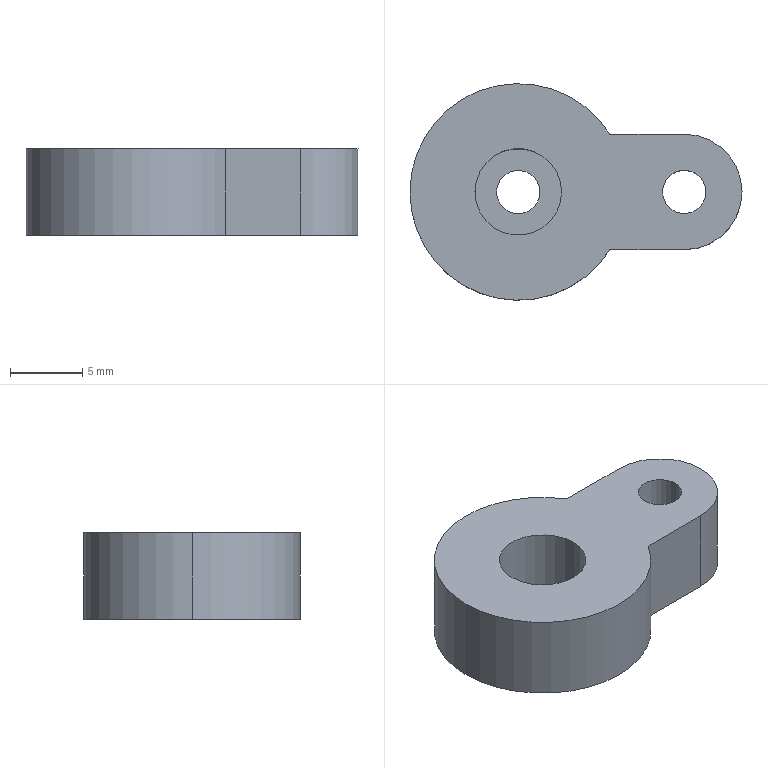Part | SolidWorks | features BaseBody 1, Cut 1 | 1 solid | 15 faces | box 23 x 15 x 6 mm | volume 1241 mm3 | cylinder 10 | plane 5 | commonest cylinder face diameters 3 x4 6 x2 8 x2 15 x2
STEP:
#1=CARTESIAN_POINT('',(-4.04,16.034,1.5));
#2=VERTEX_POINT('',#1);
#3=CARTESIAN_POINT('',(1.96,16.034,1.5));
#4=VERTEX_POINT('',#3);
#5=CARTESIAN_POINT('',(-1.04,16.034,1.5));
#6=DIRECTION('',(0.,0.,1.));
#7=DIRECTION('',(1.,0.,0.));
#8=AXIS2_PLACEMENT_3D('',#5,#6,#7);
#9=CIRCLE('',#8,3.);
#10=EDGE_CURVE('',#2,#4,#9,.T.);
#11=ORIENTED_EDGE('',*,*,#10,.F.);
#12=CARTESIAN_POINT('',(-4.04,16.034,6.));
#13=VERTEX_POINT('',#12);
#14=CARTESIAN_POINT('',(-4.04,16.034,1.5));
#15=DIRECTION('',(0.,0.,1.));
#16=VECTOR('',#15,1000.);
#17=LINE('',#14,#16);
#18=EDGE_CURVE('',#2,#13,#17,.T.);
#19=ORIENTED_EDGE('',*,*,#18,.T.);
#20=CARTESIAN_POINT('',(1.96,16.034,6.));
#21=VERTEX_POINT('',#20);
#22=CARTESIAN_POINT('',(-1.04,16.034,6.));
#23=DIRECTION('',(0.,0.,1.));
#24=DIRECTION('',(1.,0.,0.));
#25=AXIS2_PLACEMENT_3D('',#22,#23,#24);
#26=CIRCLE('',#25,3.);
#27=EDGE_CURVE('',#13,#21,#26,.T.);
#28=ORIENTED_EDGE('',*,*,#27,.T.);
#29=CARTESIAN_POINT('',(1.96,16.034,1.5));
#30=DIRECTION('',(0.,0.,1.));
#31=VECTOR('',#30,1000.);
#32=LINE('',#29,#31);
#33=EDGE_CURVE('',#4,#21,#32,.T.);
#34=ORIENTED_EDGE('',*,*,#33,.F.);
#35=EDGE_LOOP('',(#11,#19,#28,#34));
#36=FACE_OUTER_BOUND('',#35,.T.);
#37=CARTESIAN_POINT('',(-1.04,16.034,1.5));
#38=DIRECTION('',(0.,0.,1.));
#39=DIRECTION('',(1.,0.,0.));
#40=AXIS2_PLACEMENT_3D('',#37,#38,#39);
#41=CYLINDRICAL_SURFACE('',#40,3.);
#42=ADVANCED_FACE('',(#36),#41,.F.);
#43=CARTESIAN_POINT('',(-2.54,16.034,1.5));
#44=VERTEX_POINT('',#43);
#45=CARTESIAN_POINT('',(0.46,16.034,1.5));
#46=VERTEX_POINT('',#45);
#47=CARTESIAN_POINT('',(-1.04,16.034,1.5));
#48=DIRECTION('',(0.,0.,-1.));
#49=DIRECTION('',(1.,0.,0.));
#50=AXIS2_PLACEMENT_3D('',#47,#48,#49);
#51=CIRCLE('',#50,1.5);
#52=EDGE_CURVE('',#44,#46,#51,.T.);
#53=ORIENTED_EDGE('',*,*,#52,.F.);
#54=CARTESIAN_POINT('',(-2.54,16.034,0.));
#55=VERTEX_POINT('',#54);
#56=CARTESIAN_POINT('',(-2.54,16.034,6.));
#57=DIRECTION('',(0.,0.,-1.));
#58=VECTOR('',#57,1000.);
#59=LINE('',#56,#58);
#60=EDGE_CURVE('',#44,#55,#59,.T.);
#61=ORIENTED_EDGE('',*,*,#60,.T.);
#62=CARTESIAN_POINT('',(0.46,16.034,0.));
#63=VERTEX_POINT('',#62);
#64=CARTESIAN_POINT('',(-1.04,16.034,0.));
#65=DIRECTION('',(0.,0.,1.));
#66=DIRECTION('',(1.,0.,0.));
#67=AXIS2_PLACEMENT_3D('',#64,#65,#66);
#68=CIRCLE('',#67,1.5);
#69=EDGE_CURVE('',#63,#55,#68,.T.);
#70=ORIENTED_EDGE('',*,*,#69,.F.);
#71=CARTESIAN_POINT('',(0.46,16.034,6.));
#72=DIRECTION('',(0.,0.,-1.));
#73=VECTOR('',#72,1000.);
#74=LINE('',#71,#73);
#75=EDGE_CURVE('',#46,#63,#74,.T.);
#76=ORIENTED_EDGE('',*,*,#75,.F.);
#77=EDGE_LOOP('',(#53,#61,#70,#76));
#78=FACE_OUTER_BOUND('',#77,.T.);
#79=CARTESIAN_POINT('',(-1.04,16.034,6.));
#80=DIRECTION('',(0.,0.,-1.));
#81=DIRECTION('',(-1.,0.,0.));
#82=AXIS2_PLACEMENT_3D('',#79,#80,#81);
#83=CYLINDRICAL_SURFACE('',#82,1.5);
#84=ADVANCED_FACE('',(#78),#83,.F.);
#85=CARTESIAN_POINT('',(-1.04,16.034,1.5));
#86=DIRECTION('',(0.,0.,-1.));
#87=DIRECTION('',(1.,0.,0.));
#88=AXIS2_PLACEMENT_3D('',#85,#86,#87);
#89=CIRCLE('',#88,1.5);
#90=EDGE_CURVE('',#46,#44,#89,.T.);
#91=ORIENTED_EDGE('',*,*,#90,.F.);
#92=ORIENTED_EDGE('',*,*,#75,.T.);
#93=CARTESIAN_POINT('',(-1.04,16.034,0.));
#94=DIRECTION('',(0.,0.,1.));
#95=DIRECTION('',(1.,0.,0.));
#96=AXIS2_PLACEMENT_3D('',#93,#94,#95);
#97=CIRCLE('',#96,1.5);
#98=EDGE_CURVE('',#55,#63,#97,.T.);
#99=ORIENTED_EDGE('',*,*,#98,.F.);
#100=ORIENTED_EDGE('',*,*,#60,.F.);
#101=EDGE_LOOP('',(#91,#92,#99,#100));
#102=FACE_OUTER_BOUND('',#101,.T.);
#103=CARTESIAN_POINT('',(-1.04,16.034,6.));
#104=DIRECTION('',(0.,0.,-1.));
#105=DIRECTION('',(-1.,0.,0.));
#106=AXIS2_PLACEMENT_3D('',#103,#104,#105);
#107=CYLINDRICAL_SURFACE('',#106,1.5);
#108=ADVANCED_FACE('',(#102),#107,.F.);
#109=CARTESIAN_POINT('',(14.46,16.034,0.));
#110=VERTEX_POINT('',#109);
#111=CARTESIAN_POINT('',(14.46,16.034,6.));
#112=VERTEX_POINT('',#111);
#113=CARTESIAN_POINT('',(14.46,16.034,-2.));
#114=DIRECTION('',(0.,0.,1.));
#115=VECTOR('',#114,1000.);
#116=LINE('',#113,#115);
#117=EDGE_CURVE('',#110,#112,#116,.T.);
#118=ORIENTED_EDGE('',*,*,#117,.F.);
#119=CARTESIAN_POINT('',(10.46,20.034,0.));
#120=VERTEX_POINT('',#119);
#121=CARTESIAN_POINT('',(10.46,16.034,0.));
#122=DIRECTION('',(0.,0.,-1.));
#123=DIRECTION('',(1.,0.,0.));
#124=AXIS2_PLACEMENT_3D('',#121,#122,#123);
#125=CIRCLE('',#124,4.);
#126=EDGE_CURVE('',#120,#110,#125,.T.);
#127=ORIENTED_EDGE('',*,*,#126,.F.);
#128=CARTESIAN_POINT('',(10.46,20.034,6.));
#129=VERTEX_POINT('',#128);
#130=CARTESIAN_POINT('',(10.46,20.034,6.));
#131=DIRECTION('',(0.,0.,-1.));
#132=VECTOR('',#131,1000.);
#133=LINE('',#130,#132);
#134=EDGE_CURVE('',#129,#120,#133,.T.);
#135=ORIENTED_EDGE('',*,*,#134,.F.);
#136=CARTESIAN_POINT('',(10.46,16.034,6.));
#137=DIRECTION('',(0.,0.,-1.));
#138=DIRECTION('',(1.,0.,0.));
#139=AXIS2_PLACEMENT_3D('',#136,#137,#138);
#140=CIRCLE('',#139,4.);
#141=EDGE_CURVE('',#129,#112,#140,.T.);
#142=ORIENTED_EDGE('',*,*,#141,.T.);
#143=EDGE_LOOP('',(#118,#127,#135,#142));
#144=FACE_OUTER_BOUND('',#143,.T.);
#145=CARTESIAN_POINT('',(10.46,16.034,-2.));
#146=DIRECTION('',(0.,0.,1.));
#147=DIRECTION('',(1.,0.,0.));
#148=AXIS2_PLACEMENT_3D('',#145,#146,#147);
#149=CYLINDRICAL_SURFACE('',#148,4.);
#150=ADVANCED_FACE('',(#144),#149,.T.);
#151=CARTESIAN_POINT('',(8.96,16.034,0.));
#152=VERTEX_POINT('',#151);
#153=CARTESIAN_POINT('',(8.96,16.034,6.));
#154=VERTEX_POINT('',#153);
#155=CARTESIAN_POINT('',(8.96,16.034,-4.));
#156=DIRECTION('',(0.,0.,1.));
#157=VECTOR('',#156,1000.);
#158=LINE('',#155,#157);
#159=EDGE_CURVE('',#152,#154,#158,.T.);
#160=ORIENTED_EDGE('',*,*,#159,.F.);
#161=CARTESIAN_POINT('',(11.96,16.034,0.));
#162=VERTEX_POINT('',#161);
#163=CARTESIAN_POINT('',(10.46,16.034,0.));
#164=DIRECTION('',(0.,0.,1.));
#165=DIRECTION('',(1.,0.,0.));
#166=AXIS2_PLACEMENT_3D('',#163,#164,#165);
#167=CIRCLE('',#166,1.5);
#168=EDGE_CURVE('',#162,#152,#167,.T.);
#169=ORIENTED_EDGE('',*,*,#168,.F.);
#170=CARTESIAN_POINT('',(11.96,16.034,6.));
#171=VERTEX_POINT('',#170);
#172=CARTESIAN_POINT('',(11.96,16.034,-4.));
#173=DIRECTION('',(0.,0.,1.));
#174=VECTOR('',#173,1000.);
#175=LINE('',#172,#174);
#176=EDGE_CURVE('',#162,#171,#175,.T.);
#177=ORIENTED_EDGE('',*,*,#176,.T.);
#178=CARTESIAN_POINT('',(10.46,16.034,6.));
#179=DIRECTION('',(0.,0.,1.));
#180=DIRECTION('',(1.,0.,0.));
#181=AXIS2_PLACEMENT_3D('',#178,#179,#180);
#182=CIRCLE('',#181,1.5);
#183=EDGE_CURVE('',#171,#154,#182,.T.);
#184=ORIENTED_EDGE('',*,*,#183,.T.);
#185=EDGE_LOOP('',(#160,#169,#177,#184));
#186=FACE_OUTER_BOUND('',#185,.T.);
#187=CARTESIAN_POINT('',(10.46,16.034,-4.));
#188=DIRECTION('',(0.,0.,1.));
#189=DIRECTION('',(1.,0.,0.));
#190=AXIS2_PLACEMENT_3D('',#187,#188,#189);
#191=CYLINDRICAL_SURFACE('',#190,1.5);
#192=ADVANCED_FACE('',(#186),#191,.F.);
#193=CARTESIAN_POINT('',(5.304,20.034,6.));
#194=VERTEX_POINT('',#193);
#195=CARTESIAN_POINT('',(22.96,20.034,6.));
#196=DIRECTION('',(-1.,0.,0.));
#197=VECTOR('',#196,1000.);
#198=LINE('',#195,#197);
#199=EDGE_CURVE('',#129,#194,#198,.T.);
#200=ORIENTED_EDGE('',*,*,#199,.F.);
#201=ORIENTED_EDGE('',*,*,#134,.T.);
#202=CARTESIAN_POINT('',(5.304,20.034,0.));
#203=VERTEX_POINT('',#202);
#204=CARTESIAN_POINT('',(22.96,20.034,0.));
#205=DIRECTION('',(-1.,0.,0.));
#206=VECTOR('',#205,1000.);
#207=LINE('',#204,#206);
#208=EDGE_CURVE('',#120,#203,#207,.T.);
#209=ORIENTED_EDGE('',*,*,#208,.T.);
#210=CARTESIAN_POINT('',(5.304,20.034,6.));
#211=DIRECTION('',(0.,0.,-1.));
#212=VECTOR('',#211,1000.);
#213=LINE('',#210,#212);
#214=EDGE_CURVE('',#194,#203,#213,.T.);
#215=ORIENTED_EDGE('',*,*,#214,.F.);
#216=EDGE_LOOP('',(#200,#201,#209,#215));
#217=FACE_OUTER_BOUND('',#216,.T.);
#218=CARTESIAN_POINT('',(22.96,20.034,6.));
#219=DIRECTION('',(0.,-1.,0.));
#220=DIRECTION('',(0.,0.,-1.));
#221=AXIS2_PLACEMENT_3D('',#218,#219,#220);
#222=PLANE('',#221);
#223=ADVANCED_FACE('',(#217),#222,.F.);
#224=CARTESIAN_POINT('',(5.304,12.034,0.));
#225=VERTEX_POINT('',#224);
#226=CARTESIAN_POINT('',(10.46,12.034,0.));
#227=VERTEX_POINT('',#226);
#228=CARTESIAN_POINT('',(22.96,12.034,0.));
#229=DIRECTION('',(1.,0.,0.));
#230=VECTOR('',#229,1000.);
#231=LINE('',#228,#230);
#232=EDGE_CURVE('',#225,#227,#231,.T.);
#233=ORIENTED_EDGE('',*,*,#232,.T.);
#234=CARTESIAN_POINT('',(10.46,12.034,6.));
#235=VERTEX_POINT('',#234);
#236=CARTESIAN_POINT('',(10.46,12.034,-2.));
#237=DIRECTION('',(0.,0.,1.));
#238=VECTOR('',#237,1000.);
#239=LINE('',#236,#238);
#240=EDGE_CURVE('',#227,#235,#239,.T.);
#241=ORIENTED_EDGE('',*,*,#240,.T.);
#242=CARTESIAN_POINT('',(5.304,12.034,6.));
#243=VERTEX_POINT('',#242);
#244=CARTESIAN_POINT('',(22.96,12.034,6.));
#245=DIRECTION('',(1.,0.,0.));
#246=VECTOR('',#245,1000.);
#247=LINE('',#244,#246);
#248=EDGE_CURVE('',#243,#235,#247,.T.);
#249=ORIENTED_EDGE('',*,*,#248,.F.);
#250=CARTESIAN_POINT('',(5.304,12.034,6.));
#251=DIRECTION('',(0.,0.,-1.));
#252=VECTOR('',#251,1000.);
#253=LINE('',#250,#252);
#254=EDGE_CURVE('',#243,#225,#253,.T.);
#255=ORIENTED_EDGE('',*,*,#254,.T.);
#256=EDGE_LOOP('',(#233,#241,#249,#255));
#257=FACE_OUTER_BOUND('',#256,.T.);
#258=CARTESIAN_POINT('',(22.96,12.034,6.));
#259=DIRECTION('',(0.,1.,0.));
#260=DIRECTION('',(1.,0.,0.));
#261=AXIS2_PLACEMENT_3D('',#258,#259,#260);
#262=PLANE('',#261);
#263=ADVANCED_FACE('',(#257),#262,.F.);
#264=CARTESIAN_POINT('',(-8.54,16.034,6.));
#265=VERTEX_POINT('',#264);
#266=CARTESIAN_POINT('',(-8.54,16.034,0.));
#267=VERTEX_POINT('',#266);
#268=CARTESIAN_POINT('',(-8.54,16.034,6.));
#269=DIRECTION('',(0.,0.,-1.));
#270=VECTOR('',#269,1000.);
#271=LINE('',#268,#270);
#272=EDGE_CURVE('',#265,#267,#271,.T.);
#273=ORIENTED_EDGE('',*,*,#272,.F.);
#274=CARTESIAN_POINT('',(-1.04,16.034,6.));
#275=DIRECTION('',(0.,0.,1.));
#276=DIRECTION('',(1.,0.,0.));
#277=AXIS2_PLACEMENT_3D('',#274,#275,#276);
#278=CIRCLE('',#277,7.5);
#279=EDGE_CURVE('',#194,#265,#278,.T.);
#280=ORIENTED_EDGE('',*,*,#279,.F.);
#281=ORIENTED_EDGE('',*,*,#214,.T.);
#282=CARTESIAN_POINT('',(-1.04,16.034,0.));
#283=DIRECTION('',(0.,0.,1.));
#284=DIRECTION('',(1.,0.,0.));
#285=AXIS2_PLACEMENT_3D('',#282,#283,#284);
#286=CIRCLE('',#285,7.5);
#287=EDGE_CURVE('',#203,#267,#286,.T.);
#288=ORIENTED_EDGE('',*,*,#287,.T.);
#289=EDGE_LOOP('',(#273,#280,#281,#288));
#290=FACE_OUTER_BOUND('',#289,.T.);
#291=CARTESIAN_POINT('',(-1.04,16.034,6.));
#292=DIRECTION('',(0.,0.,-1.));
#293=DIRECTION('',(-1.,0.,0.));
#294=AXIS2_PLACEMENT_3D('',#291,#292,#293);
#295=CYLINDRICAL_SURFACE('',#294,7.5);
#296=ADVANCED_FACE('',(#290),#295,.T.);
#297=ORIENTED_EDGE('',*,*,#98,.T.);
#298=ORIENTED_EDGE('',*,*,#69,.T.);
#299=EDGE_LOOP('',(#297,#298));
#300=FACE_BOUND('',#299,.T.);
#301=ORIENTED_EDGE('',*,*,#168,.T.);
#302=CARTESIAN_POINT('',(10.46,16.034,0.));
#303=DIRECTION('',(0.,0.,1.));
#304=DIRECTION('',(1.,0.,0.));
#305=AXIS2_PLACEMENT_3D('',#302,#303,#304);
#306=CIRCLE('',#305,1.5);
#307=EDGE_CURVE('',#152,#162,#306,.T.);
#308=ORIENTED_EDGE('',*,*,#307,.T.);
#309=EDGE_LOOP('',(#301,#308));
#310=FACE_BOUND('',#309,.T.);
#311=ORIENTED_EDGE('',*,*,#208,.F.);
#312=ORIENTED_EDGE('',*,*,#126,.T.);
#313=CARTESIAN_POINT('',(10.46,16.034,0.));
#314=DIRECTION('',(0.,0.,-1.));
#315=DIRECTION('',(1.,0.,0.));
#316=AXIS2_PLACEMENT_3D('',#313,#314,#315);
#317=CIRCLE('',#316,4.);
#318=EDGE_CURVE('',#110,#227,#317,.T.);
#319=ORIENTED_EDGE('',*,*,#318,.T.);
#320=ORIENTED_EDGE('',*,*,#232,.F.);
#321=CARTESIAN_POINT('',(-1.04,16.034,0.));
#322=DIRECTION('',(0.,0.,1.));
#323=DIRECTION('',(1.,0.,0.));
#324=AXIS2_PLACEMENT_3D('',#321,#322,#323);
#325=CIRCLE('',#324,7.5);
#326=EDGE_CURVE('',#267,#225,#325,.T.);
#327=ORIENTED_EDGE('',*,*,#326,.F.);
#328=ORIENTED_EDGE('',*,*,#287,.F.);
#329=EDGE_LOOP('',(#311,#312,#319,#320,#327,#328));
#330=FACE_OUTER_BOUND('',#329,.T.);
#331=CARTESIAN_POINT('',(-1.04,16.034,0.));
#332=DIRECTION('',(0.,0.,1.));
#333=DIRECTION('',(1.,0.,0.));
#334=AXIS2_PLACEMENT_3D('',#331,#332,#333);
#335=PLANE('',#334);
#336=ADVANCED_FACE('',(#300,#310,#330),#335,.F.);
#337=CARTESIAN_POINT('',(-1.04,16.034,6.));
#338=DIRECTION('',(0.,0.,1.));
#339=DIRECTION('',(1.,0.,0.));
#340=AXIS2_PLACEMENT_3D('',#337,#338,#339);
#341=CIRCLE('',#340,3.);
#342=EDGE_CURVE('',#21,#13,#341,.T.);
#343=ORIENTED_EDGE('',*,*,#342,.F.);
#344=ORIENTED_EDGE('',*,*,#27,.F.);
#345=EDGE_LOOP('',(#343,#344));
#346=FACE_BOUND('',#345,.T.);
#347=ORIENTED_EDGE('',*,*,#183,.F.);
#348=CARTESIAN_POINT('',(10.46,16.034,6.));
#349=DIRECTION('',(0.,0.,1.));
#350=DIRECTION('',(1.,0.,0.));
#351=AXIS2_PLACEMENT_3D('',#348,#349,#350);
#352=CIRCLE('',#351,1.5);
#353=EDGE_CURVE('',#154,#171,#352,.T.);
#354=ORIENTED_EDGE('',*,*,#353,.F.);
#355=EDGE_LOOP('',(#347,#354));
#356=FACE_BOUND('',#355,.T.);
#357=ORIENTED_EDGE('',*,*,#141,.F.);
#358=ORIENTED_EDGE('',*,*,#199,.T.);
#359=ORIENTED_EDGE('',*,*,#279,.T.);
#360=CARTESIAN_POINT('',(-1.04,16.034,6.));
#361=DIRECTION('',(0.,0.,1.));
#362=DIRECTION('',(1.,0.,0.));
#363=AXIS2_PLACEMENT_3D('',#360,#361,#362);
#364=CIRCLE('',#363,7.5);
#365=EDGE_CURVE('',#265,#243,#364,.T.);
#366=ORIENTED_EDGE('',*,*,#365,.T.);
#367=ORIENTED_EDGE('',*,*,#248,.T.);
#368=CARTESIAN_POINT('',(10.46,16.034,6.));
#369=DIRECTION('',(0.,0.,-1.));
#370=DIRECTION('',(1.,0.,0.));
#371=AXIS2_PLACEMENT_3D('',#368,#369,#370);
#372=CIRCLE('',#371,4.);
#373=EDGE_CURVE('',#112,#235,#372,.T.);
#374=ORIENTED_EDGE('',*,*,#373,.F.);
#375=EDGE_LOOP('',(#357,#358,#359,#366,#367,#374));
#376=FACE_OUTER_BOUND('',#375,.T.);
#377=CARTESIAN_POINT('',(-1.04,16.034,6.));
#378=DIRECTION('',(0.,0.,1.));
#379=DIRECTION('',(1.,0.,0.));
#380=AXIS2_PLACEMENT_3D('',#377,#378,#379);
#381=PLANE('',#380);
#382=ADVANCED_FACE('',(#346,#356,#376),#381,.T.);
#383=ORIENTED_EDGE('',*,*,#365,.F.);
#384=ORIENTED_EDGE('',*,*,#272,.T.);
#385=ORIENTED_EDGE('',*,*,#326,.T.);
#386=ORIENTED_EDGE('',*,*,#254,.F.);
#387=EDGE_LOOP('',(#383,#384,#385,#386));
#388=FACE_OUTER_BOUND('',#387,.T.);
#389=CARTESIAN_POINT('',(-1.04,16.034,6.));
#390=DIRECTION('',(0.,0.,-1.));
#391=DIRECTION('',(-1.,0.,0.));
#392=AXIS2_PLACEMENT_3D('',#389,#390,#391);
#393=CYLINDRICAL_SURFACE('',#392,7.5);
#394=ADVANCED_FACE('',(#388),#393,.T.);
#395=ORIENTED_EDGE('',*,*,#307,.F.);
#396=ORIENTED_EDGE('',*,*,#159,.T.);
#397=ORIENTED_EDGE('',*,*,#353,.T.);
#398=ORIENTED_EDGE('',*,*,#176,.F.);
#399=EDGE_LOOP('',(#395,#396,#397,#398));
#400=FACE_OUTER_BOUND('',#399,.T.);
#401=CARTESIAN_POINT('',(10.46,16.034,-4.));
#402=DIRECTION('',(0.,0.,1.));
#403=DIRECTION('',(1.,0.,0.));
#404=AXIS2_PLACEMENT_3D('',#401,#402,#403);
#405=CYLINDRICAL_SURFACE('',#404,1.5);
#406=ADVANCED_FACE('',(#400),#405,.F.);
#407=ORIENTED_EDGE('',*,*,#318,.F.);
#408=ORIENTED_EDGE('',*,*,#117,.T.);
#409=ORIENTED_EDGE('',*,*,#373,.T.);
#410=ORIENTED_EDGE('',*,*,#240,.F.);
#411=EDGE_LOOP('',(#407,#408,#409,#410));
#412=FACE_OUTER_BOUND('',#411,.T.);
#413=CARTESIAN_POINT('',(10.46,16.034,-2.));
#414=DIRECTION('',(0.,0.,1.));
#415=DIRECTION('',(1.,0.,0.));
#416=AXIS2_PLACEMENT_3D('',#413,#414,#415);
#417=CYLINDRICAL_SURFACE('',#416,4.);
#418=ADVANCED_FACE('',(#412),#417,.T.);
#419=CARTESIAN_POINT('',(-1.04,16.034,1.5));
#420=DIRECTION('',(0.,0.,1.));
#421=DIRECTION('',(1.,0.,0.));
#422=AXIS2_PLACEMENT_3D('',#419,#420,#421);
#423=CIRCLE('',#422,3.);
#424=EDGE_CURVE('',#4,#2,#423,.T.);
#425=ORIENTED_EDGE('',*,*,#424,.T.);
#426=ORIENTED_EDGE('',*,*,#10,.T.);
#427=EDGE_LOOP('',(#425,#426));
#428=FACE_OUTER_BOUND('',#427,.T.);
#429=ORIENTED_EDGE('',*,*,#52,.T.);
#430=ORIENTED_EDGE('',*,*,#90,.T.);
#431=EDGE_LOOP('',(#429,#430));
#432=FACE_BOUND('',#431,.T.);
#433=CARTESIAN_POINT('',(-1.04,16.034,1.5));
#434=DIRECTION('',(0.,0.,1.));
#435=DIRECTION('',(1.,0.,0.));
#436=AXIS2_PLACEMENT_3D('',#433,#434,#435);
#437=PLANE('',#436);
#438=ADVANCED_FACE('',(#428,#432),#437,.T.);
#439=ORIENTED_EDGE('',*,*,#18,.F.);
#440=ORIENTED_EDGE('',*,*,#424,.F.);
#441=ORIENTED_EDGE('',*,*,#33,.T.);
#442=ORIENTED_EDGE('',*,*,#342,.T.);
#443=EDGE_LOOP('',(#439,#440,#441,#442));
#444=FACE_OUTER_BOUND('',#443,.T.);
#445=CARTESIAN_POINT('',(-1.04,16.034,1.5));
#446=DIRECTION('',(0.,0.,1.));
#447=DIRECTION('',(1.,0.,0.));
#448=AXIS2_PLACEMENT_3D('',#445,#446,#447);
#449=CYLINDRICAL_SURFACE('',#448,3.);
#450=ADVANCED_FACE('',(#444),#449,.F.);
#451=CLOSED_SHELL('',(#42,#84,#108,#150,#192,#223,#263,#296,#336,#382,#394,#406,#418,#438,#450));
#452=MANIFOLD_SOLID_BREP('',#451);
#453=CARTESIAN_POINT('',(0.,0.,0.));
#454=DIRECTION('',(0.,0.,1.));
#455=DIRECTION('',(1.,0.,0.));
#456=AXIS2_PLACEMENT_3D('',#453,#454,#455);
#457=(LENGTH_UNIT()NAMED_UNIT(*)SI_UNIT(.MILLI.,.METRE.));
#458=UNCERTAINTY_MEASURE_WITH_UNIT(LENGTH_MEASURE(0.00001),#457,'','');
#459=(NAMED_UNIT(*)PLANE_ANGLE_UNIT()SI_UNIT($,.RADIAN.));
#460=(NAMED_UNIT(*)SI_UNIT($,.STERADIAN.)SOLID_ANGLE_UNIT());
#461=(GEOMETRIC_REPRESENTATION_CONTEXT(3)GLOBAL_UNCERTAINTY_ASSIGNED_CONTEXT((#458))GLOBAL_UNIT_ASSIGNED_CONTEXT((#457,#459,#460))REPRESENTATION_CONTEXT('',''));
#462=ADVANCED_BREP_SHAPE_REPRESENTATION('',(#452,#456),#461);